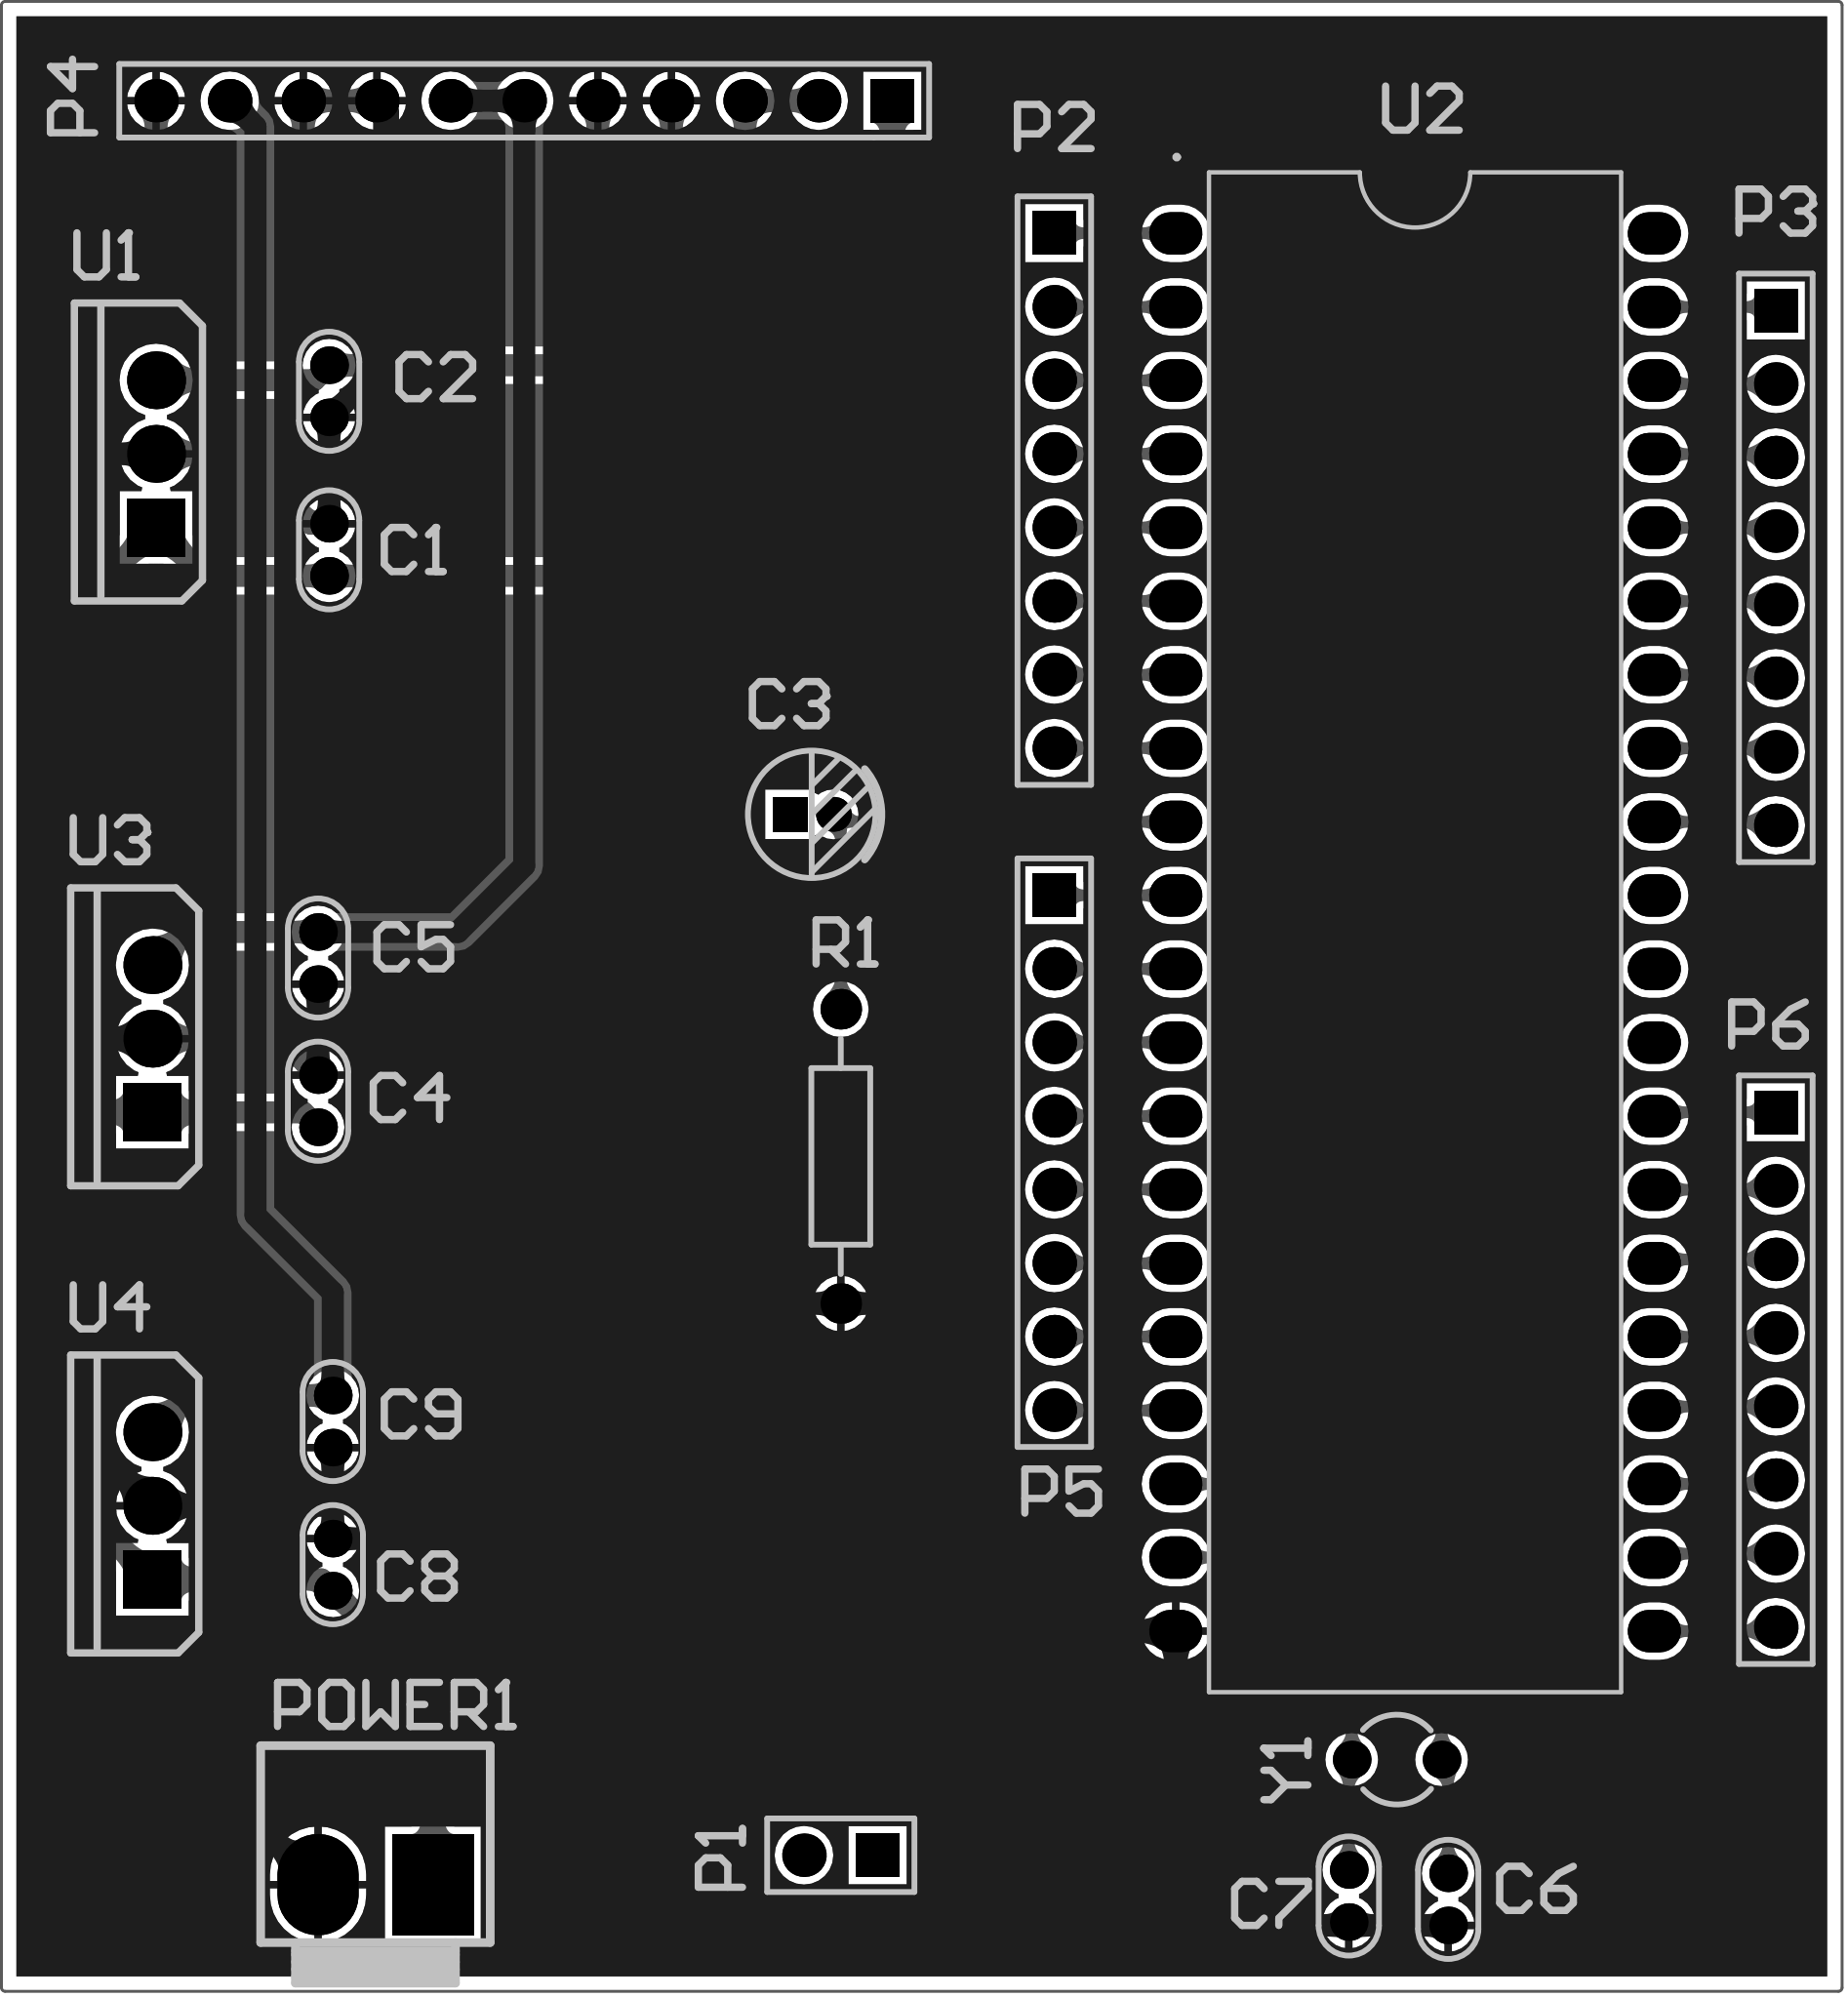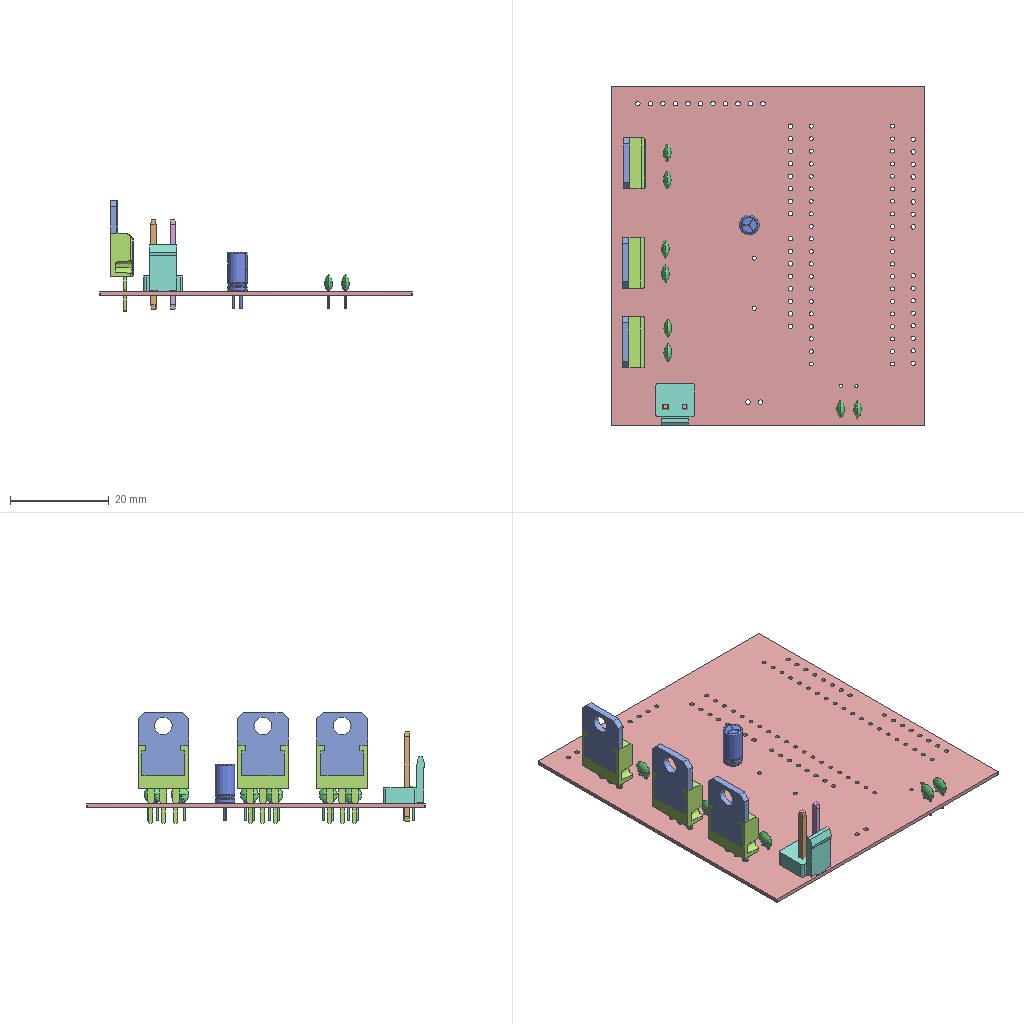Circuit board layout | Altium Designer | box 63.5 x 68.7 x 22.5 mm
Layer stack:
# Altium Designer layer stack of  (unit mm; dielectric type: 0 none, 1 core, 2 prepreg, 3 surface material)
index,name,kind,layer,copper_thickness_mm,dielectric_type,dielectric_thickness_mm,dielectric_material,dielectric_constant
0,Top Paste,other,,,,,,
1,Top Overlay,other,,,,,,
2,Top Solder,dielectric,,,3,0.0102,Solder Resist,3.5
3,Top Layer,copper,Top Layer,0.0356,,,,
4,Dielectric 1,dielectric,,,1,0.254,FR-4,4.2
5,GND,copper,GND,0.036,,,,
6,Dielectric 3,dielectric,,,2,0.127,,4.2
7,VCC,copper,VCC,0.036,,,,
8,Dielectric 2,dielectric,,,1,0.254,,4.2
9,Bottom Layer,copper,Bottom Layer,0.0356,,,,
10,Bottom Solder,dielectric,,,3,0.0102,Solder Resist,3.5
11,Bottom Overlay,other,,,,,,
12,Bottom Paste,other,,,,,,
# drill layer pairs: low layer,high layer
drill_pair,Top Layer,Bottom Layer
Part placement:
Designator,Comment,Layer,Footprint,Center-X(mm),Center-Y(mm),Rotation
Y1,XTAL,TopLayer,R38,93.599,30.226,90
U4,7806,TopLayer,TO220A,50.673,38.989,90
U3,7805,TopLayer,TO220A,50.673,55.118,90
U2,STC89C52RC,TopLayer,STC89C52RC,94.234,58.793,270
U1,7805,TopLayer,TO220A,50.8,75.311,90
R1,10K,TopLayer,AXIAL-0.4,74.422,51.054,90
POWER1,Terminal block,TopLayer,VH3.96-2A,58.368,25.908,180
P6,Header 8,TopLayer,HDR1X8,106.68,43.688,270
P5,Header 8,TopLayer,HDR1X8,81.788,51.181,270
P4,Header 11,TopLayer,HDR1X11,63.5,87.503,180
P3,Header 8,TopLayer,HDR1X8,106.68,71.374,270
P2,Header 8,TopLayer,HDR1X8,81.788,74.041,270
P1,Header 2,TopLayer,HDR1X2,74.422,26.924,180
C9,0.1UF,TopLayer,CC_1.8*3.6,56.896,41.899,270
C8,0.33UF,TopLayer,CC_1.8*3.6,56.896,36.957,90
C7,22pF,TopLayer,CC_1.8*3.6,91.948,25.516,270
C6,22pF,TopLayer,CC_1.8*3.6,95.377,25.4,270
C5,0.1UF,TopLayer,CC_1.8*3.6,56.388,57.901,270
C4,0.33UF,TopLayer,CC_1.8*3.6,56.388,52.959,90
C3,10UF,TopLayer,CAP_1.5*4*8,73.418,62.865,0
C2,0.1UF,TopLayer,CC_1.8*3.6,56.769,77.47,270
C1,0.33UF,TopLayer,CC_1.8*3.6,56.769,71.998,90
Pad and via stacks:
# Altium Designer via and pad stacks of  (unit mm). Each distinct definition once, with the count of objects using it.
# via: kind,start_layer,end_layer,hole_mm,diameter_mm,mode(0 simple;1 top-mid-bottom;2 full stack),diameter_per_layer,count,example_net
# pad: kind,layer,hole_mm,hole_type(0 round;1 square;2 slot),plating,top_size,top_shape(1 round;2 rect;3 octagon;9 rounded rect),mid_size,bottom_size,mode,footprint,size_per_layer,count,example
pad,Multi-Layer,0.9,0,plated,1.5x1.5,2,1.5x1.5,1.5x1.5,0,HDR1X8,,4,P3.1
pad,Multi-Layer,0.9,0,plated,1.5x1.5,1,1.5x1.5,1.5x1.5,0,HDR1X8,,28,P3.2
pad,Multi-Layer,0.5,0,plated,1.3x1.3,1,1.3x1.3,1.3x1.3,0,CC 1.8*3.6,,16,C2.2
pad,Multi-Layer,1.1,0,plated,2x2,1,2x2,2x2,0,TO220A,,6,U3.2
pad,Multi-Layer,1.1,0,plated,2x2,2,2x2,2x2,0,TO220A,,3,U3.1
pad,Multi-Layer,0.6,0,plated,1.2x1.2,1,1.2x1.2,1.2x1.2,0,CAP 1.5*4*8,,1,C3.2
pad,Multi-Layer,0.6,0,plated,1.2x1.2,2,1.2x1.2,1.2x1.2,0,CAP 1.5*4*8,,1,C3.1
pad,Multi-Layer,0.9,0,plated,1.5x1.5,2,1.5x1.5,1.5x1.5,0,HDR1X2,,1,P1.1
pad,Multi-Layer,0.9,0,plated,1.5x1.5,1,1.5x1.5,1.5x1.5,0,HDR1X2,,1,P1.2
pad,Multi-Layer,0.9,0,plated,1.5x1.5,1,1.5x1.5,1.5x1.5,0,HDR1X11,,10,P4.11
pad,Multi-Layer,0.9,0,plated,1.5x1.5,2,1.5x1.5,1.5x1.5,0,HDR1X11,,1,P4.1
pad,Multi-Layer,1.6,0,plated,2.8x3.5,2,2.8x3.5,2.8x3.5,0,VH3.96-2A,,1,POWER1.1
pad,Multi-Layer,1.6,0,plated,2.8x3.5,1,2.8x3.5,2.8x3.5,0,VH3.96-2A,,1,POWER1.2
pad,Multi-Layer,0.85,0,plated,1.4x1.4,1,1.4x1.4,1.4x1.4,0,AXIAL-0.4,,2,R1.1
pad,Multi-Layer,0.8,0,plated,1.467x1.833,1,1.467x1.833,1.467x1.833,0,STC89C52RC,,40,U2.1
pad,Multi-Layer,0.7,0,plated,1.3x1.3,1,1.3x1.3,1.3x1.3,0,R38,,2,Y1.1
Copper pours:
name,layer,net,type(0 solid;1 hatched;2 none)
D,Top Layer,GND,0
D,Bottom Layer,GND,0
Design rules, without the lines most boards share:
# Altium Designer design rules of  (exported by Altium Designer, unit mm)
# columns: name | kind | enabled | priority | scope1 | scope2 | descriptor | typed fields (field=value)
SilkToSilkClearance | 55 | enabled | 1 | All | All | Silk to Silk (Clearance=0mil) (All),(All) |
SilkToSolderMaskClearance | 54 | enabled | 1 | IsPad | All | Silk To Solder Mask (Clearance=0mil) (IsPad),(All) |
MinimumSolderMaskSliver | 53 | enabled | 1 | All | All | Minimum Solder Mask Sliver (Gap=0mil) (All),(All) |
HoleToHoleClearance | 52 | enabled | 1 | All | All | Hole To Hole Clearance (Gap=10mil) (All),(All) | gap=0.254
DiffPairsRouting | 51 | enabled | 1 | All | All | Differential Pairs Uncoupled Length using the Gap Constraints (Min=10mil) (Max=10mil) (Prefered=10mil)  and Width Constraints (Min=15mil) (Max=15mil) (Prefered=15mil) (All) |
SolderMaskExpansion | 13 | enabled | 1 | All | All | Solder Mask Expansion (Expansion =4mil) (All) | expansion=0.1016
RoutingVias | 11 | enabled | 1 | All | All | Routing Via (MinHoleWidth=28mil) (MaxHoleWidth=28mil) (PreferredHoleWidth=28mil) (MinWidth=50mil) (MaxWidth=50mil) (PreferedWidth=50mil) (All) | via_min_hole=0.7112 via_max_hole=0.7112 via_preferred_diameter=1.27 via_preferred_hole=0.7112
Width | 2 | enabled | 1 | All | All | Width Constraint (Min=15mil) (Max=30mil) (Preferred=15mil) (All) |
PolygonConnect | 20 | enabled | 1 | All | All | Polygon Connect Rule(Relief Connect )(Conductor Width=10mil) (Relief Angle=90 Angle) (Entries=4) (Air Gap Width=10mil) (All),(All) | connect_style(0=relief,1=direct,2=none)=0 relief_conductor_width=0.254 relief_entries=4
PlaneConnect | 6 | enabled | 1 | All | All | Power Plane Connect Rule(Relief Connect )(Expansion=20mil) (Conductor Width=10mil) (Air Gap=10mil) (Entries=4) (All) | relief_conductor_width=0.254 relief_entries=4 relief_expansion=0.508
Clearance | 0 | enabled | 1 | All | All | Clearance Constraint (Gap=10mil) (All),(All) | gap=0.254
Classes set for this board:
# Altium Designer classes of  (member kind: 0 net, 1 component, 2 from-to, 3 pad, 4 layer, 5 differential pair, 6 design channel, 7 polygon, 8 structure, 9 xSignal)
# columns: class name | member kind | superclass | members
Sheet2 | 1 | no | C1; C2; C3; C4; C5; C6; C7; C8; C9; P1; P2; P3; P4; P5; P6; POWER1; R1; U1; U2; U3; U4; Y1;